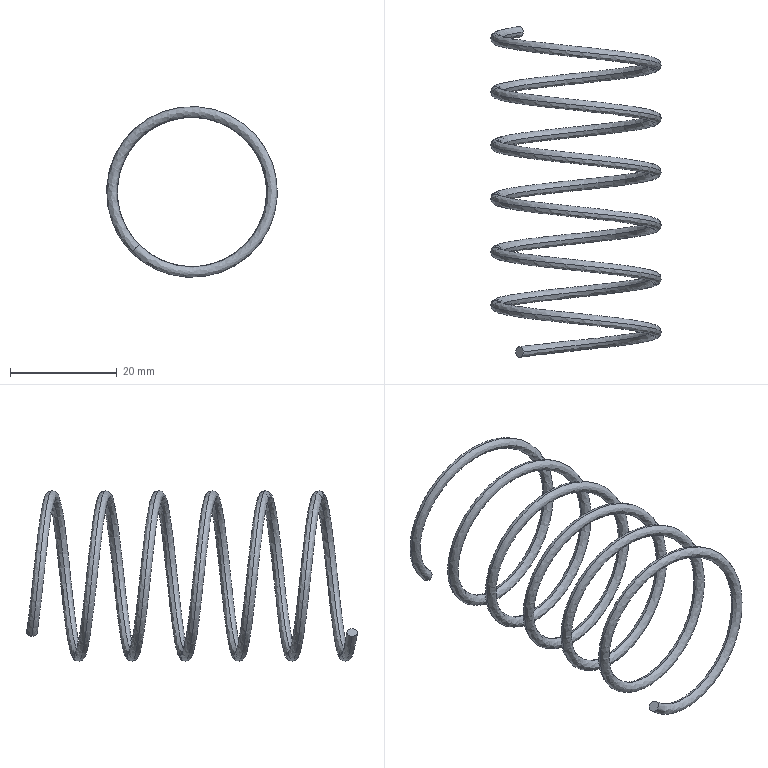Part | STEP file | Lo xo bac truot | 1 solid | 4 faces | box 32 x 62 x 32 mm | volume 1777 mm3 | spline 2 | plane 2